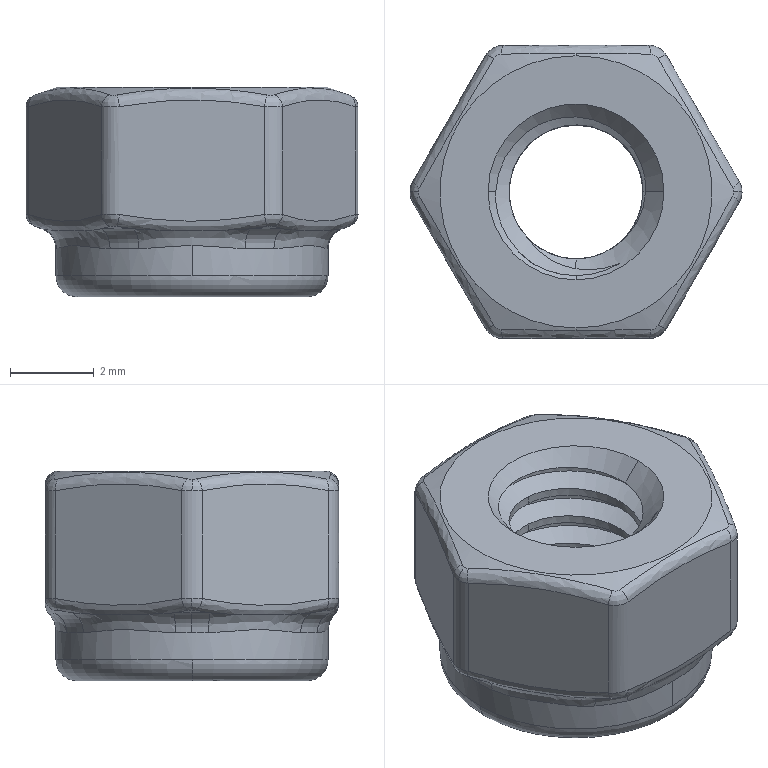Part | SolidWorks | features BaseBody 1 | 1 solid | 94 faces | volume 142.46 mm3 | spline 40 | cylinder 22 | cone 12 | plane 10 | torus 10 | commonest cylinder face diameters 3.2 x10 1 x8 5 x2 6.5 x2